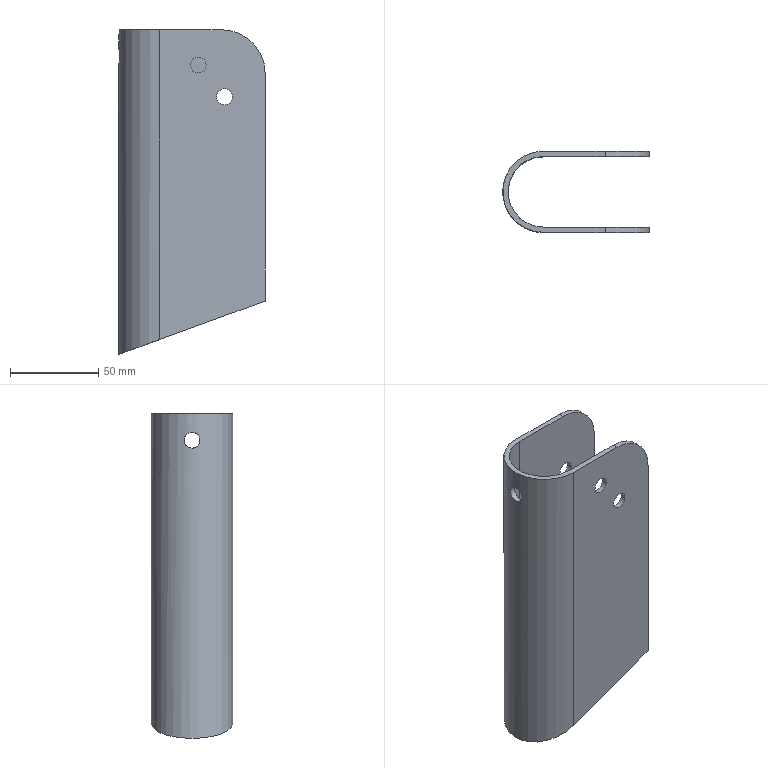Part | STEP file | 5090103L | 1 solid | 16 faces | box 83 x 46 x 184 mm | volume 94323 mm3 | cylinder 8 | plane 8 | commonest cylinder face diameters 9 x4 50 x2 40 x1 46 x1